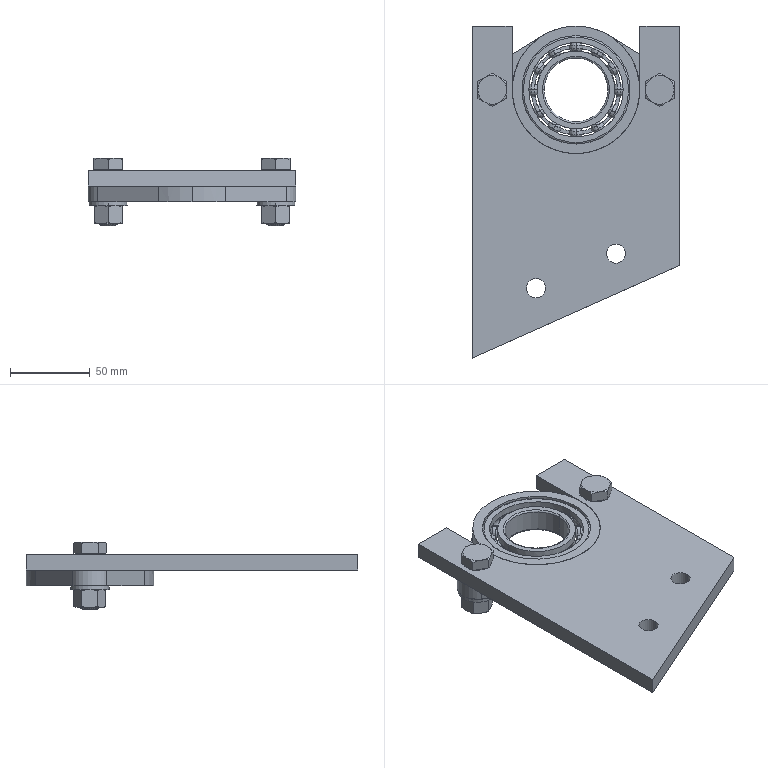Part | SolidWorks | features CompositeCurve 1 | 9 solids | 433 faces | box 130 x 208 x 42.5 mm | volume 256605 mm3 | cone 136 | plane 96 | sphere 96 | cylinder 57 | torus 48 | commonest cylinder face diameters 12 x20 13 x4 18 x4 24 x4 48.8 x4 59.2 x4